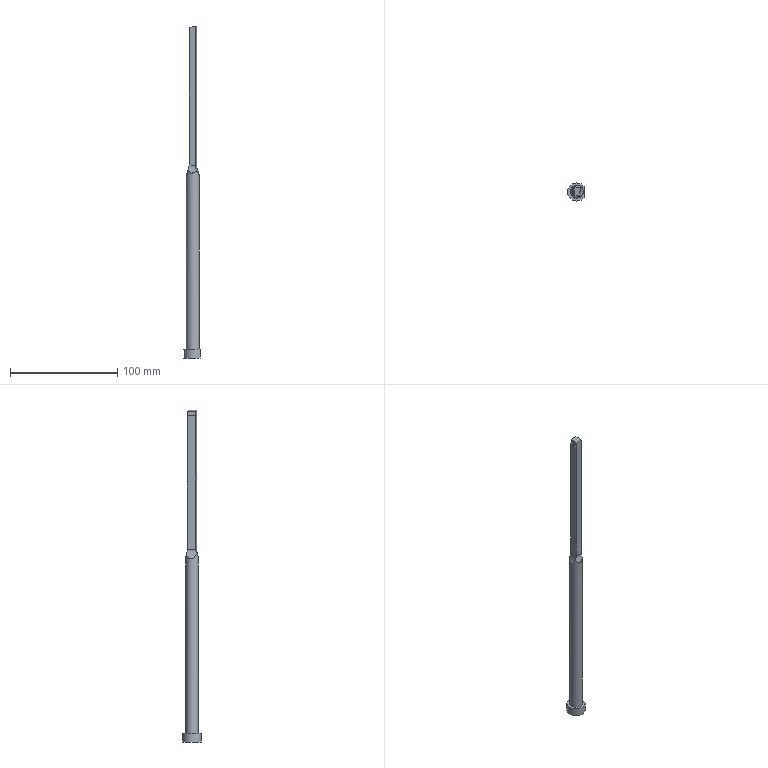Part | STEP file | D17XH8Xd12XA6XB8X310LXN180 | 1 solid | 16 faces | box 15.5 x 17 x 309.851 mm | volume 27016 mm3 | spline 7 | plane 5 | cylinder 4 | commonest cylinder face diameters 30 x2 12 x1 17 x1